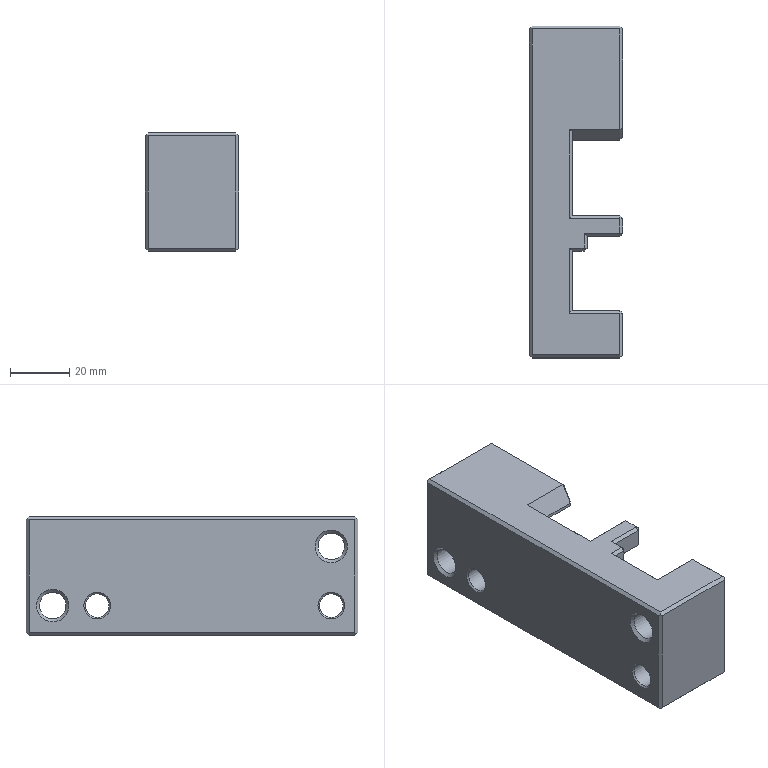Part | NX | features BREP 8, CHAMFER 2, solid 2, SUBTRACT 1 | 1 solid | 195 faces | box 31.5 x 112 x 40 mm | volume 86589 mm3 | plane 121 | spline 46 | cone 18 | cylinder 10 | commonest cylinder face diameters 6 x4 8 x2 9 x2 10.5 x2